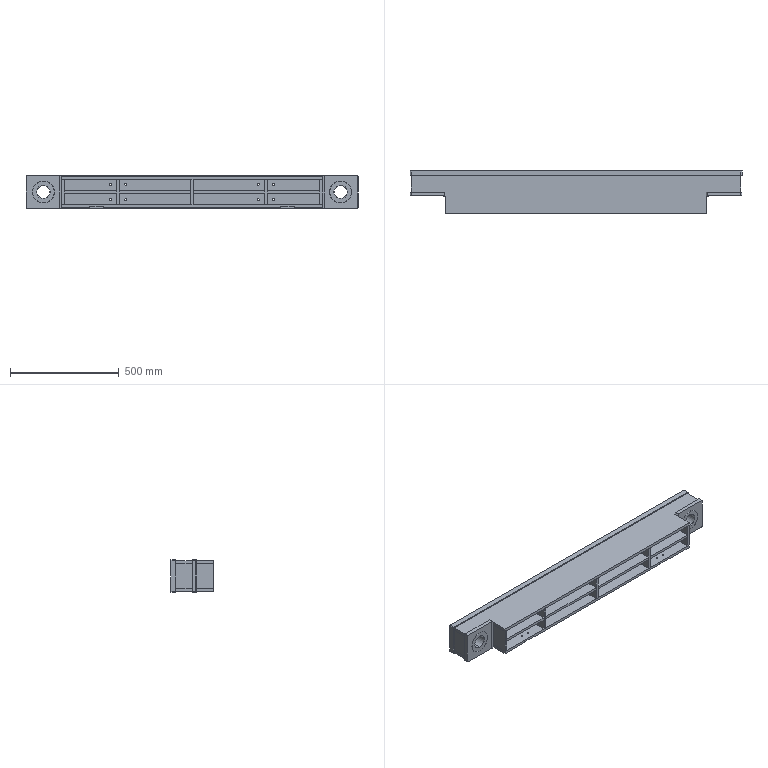Part | SolidWorks | 18 solids | 230 faces | box 1530 x 195 x 150 mm | volume 16687535 mm3 | plane 148 | cylinder 70 | cone 12 | commonest cylinder face diameters 10 x18 6.8 x16 10.2 x16 60 x8 80 x4 100 x4